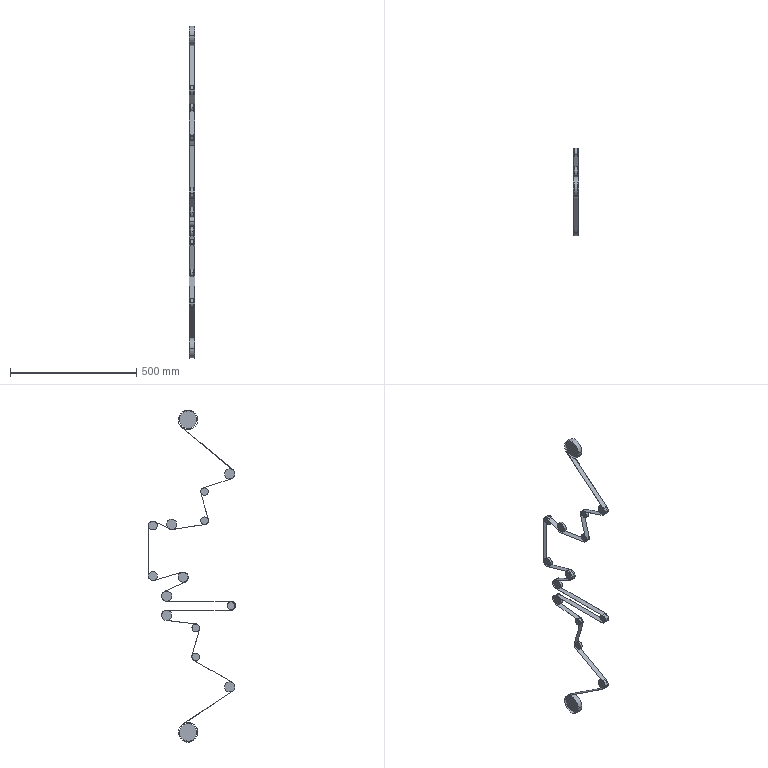Part | STEP file | Tape feed wrap diagram | 16 solids | 144 faces | box 20 x 346.75 x 1318 mm | volume 219879 mm3 | cylinder 80 | plane 64 | commonest cylinder face diameters 40 x12 30 x10 41 x9 41.4 x7 31 x6 77.5 x6